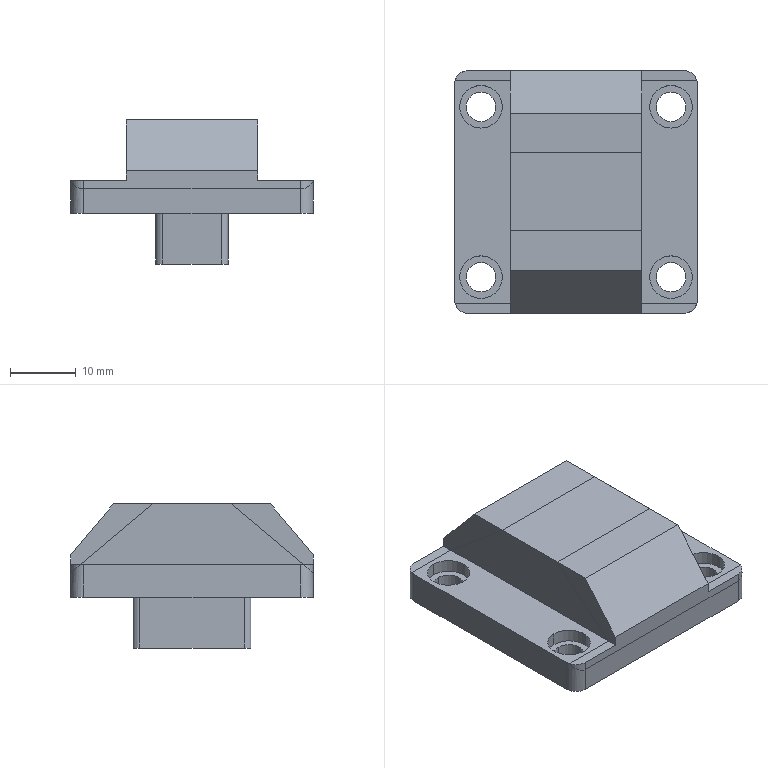Part | 2 solids | 116 faces | box 37 x 37 x 22 mm | volume 24262 mm3 | cylinder 62 | plane 42 | cone 12 | commonest cylinder face diameters 4.5 x16 6.5 x16 6 x10 2 x8 4 x8 8.8 x4